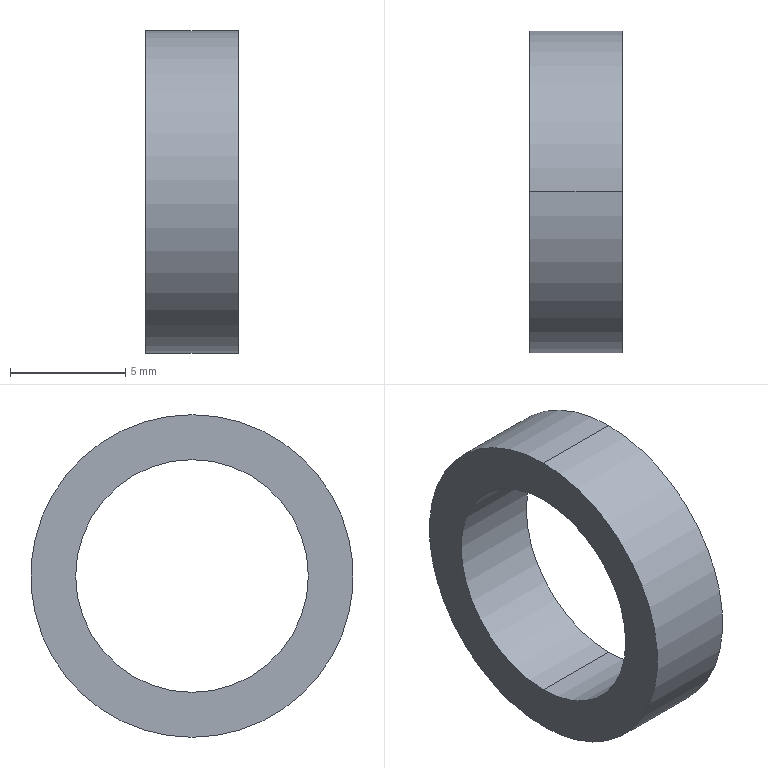Part | SolidWorks | features BaseBody 1 | 1 solid | 6 faces | box 4 x 14 x 14 mm | volume 295.278 mm3 | cylinder 4 | plane 2 | commonest cylinder face diameters 10.1 x2 14 x2
STEP:
#1=CARTESIAN_POINT('',(-2.,0.,-7.));
#2=VERTEX_POINT('',#1);
#3=CARTESIAN_POINT('',(-2.,0.,7.));
#4=VERTEX_POINT('',#3);
#5=CARTESIAN_POINT('',(-2.,0.,0.));
#6=DIRECTION('',(1.,0.,0.));
#7=DIRECTION('',(0.,0.,-1.));
#8=AXIS2_PLACEMENT_3D('',#5,#6,#7);
#9=CIRCLE('',#8,7.);
#10=EDGE_CURVE('',#2,#4,#9,.T.);
#11=ORIENTED_EDGE('',*,*,#10,.T.);
#12=CARTESIAN_POINT('',(2.,0.,7.));
#13=VERTEX_POINT('',#12);
#14=CARTESIAN_POINT('',(-2.,0.,7.));
#15=DIRECTION('',(1.,0.,0.));
#16=VECTOR('',#15,1000.);
#17=LINE('',#14,#16);
#18=EDGE_CURVE('',#4,#13,#17,.T.);
#19=ORIENTED_EDGE('',*,*,#18,.T.);
#20=CARTESIAN_POINT('',(2.,0.,-7.));
#21=VERTEX_POINT('',#20);
#22=CARTESIAN_POINT('',(2.,0.,0.));
#23=DIRECTION('',(-1.,0.,0.));
#24=DIRECTION('',(0.,0.,-1.));
#25=AXIS2_PLACEMENT_3D('',#22,#23,#24);
#26=CIRCLE('',#25,7.);
#27=EDGE_CURVE('',#13,#21,#26,.T.);
#28=ORIENTED_EDGE('',*,*,#27,.T.);
#29=CARTESIAN_POINT('',(-2.,0.,-7.));
#30=DIRECTION('',(1.,0.,0.));
#31=VECTOR('',#30,1000.);
#32=LINE('',#29,#31);
#33=EDGE_CURVE('',#2,#21,#32,.T.);
#34=ORIENTED_EDGE('',*,*,#33,.F.);
#35=EDGE_LOOP('',(#11,#19,#28,#34));
#36=FACE_OUTER_BOUND('',#35,.T.);
#37=CARTESIAN_POINT('',(-2.,0.,0.));
#38=DIRECTION('',(1.,0.,0.));
#39=DIRECTION('',(0.,0.,-1.));
#40=AXIS2_PLACEMENT_3D('',#37,#38,#39);
#41=CYLINDRICAL_SURFACE('',#40,7.);
#42=ADVANCED_FACE('',(#36),#41,.T.);
#43=CARTESIAN_POINT('',(-2.,0.,-5.05));
#44=VERTEX_POINT('',#43);
#45=CARTESIAN_POINT('',(-2.,0.,5.05));
#46=VERTEX_POINT('',#45);
#47=CARTESIAN_POINT('',(-2.,0.,0.));
#48=DIRECTION('',(-1.,0.,0.));
#49=DIRECTION('',(0.,0.,-1.));
#50=AXIS2_PLACEMENT_3D('',#47,#48,#49);
#51=CIRCLE('',#50,5.05);
#52=EDGE_CURVE('',#44,#46,#51,.T.);
#53=ORIENTED_EDGE('',*,*,#52,.T.);
#54=CARTESIAN_POINT('',(2.,0.,5.05));
#55=VERTEX_POINT('',#54);
#56=CARTESIAN_POINT('',(-3.,0.,5.05));
#57=DIRECTION('',(1.,0.,0.));
#58=VECTOR('',#57,1000.);
#59=LINE('',#56,#58);
#60=EDGE_CURVE('',#46,#55,#59,.T.);
#61=ORIENTED_EDGE('',*,*,#60,.T.);
#62=CARTESIAN_POINT('',(2.,0.,-5.05));
#63=VERTEX_POINT('',#62);
#64=CARTESIAN_POINT('',(2.,0.,0.));
#65=DIRECTION('',(-1.,0.,0.));
#66=DIRECTION('',(0.,0.,-1.));
#67=AXIS2_PLACEMENT_3D('',#64,#65,#66);
#68=CIRCLE('',#67,5.05);
#69=EDGE_CURVE('',#63,#55,#68,.T.);
#70=ORIENTED_EDGE('',*,*,#69,.F.);
#71=CARTESIAN_POINT('',(-3.,0.,-5.05));
#72=DIRECTION('',(1.,0.,0.));
#73=VECTOR('',#72,1000.);
#74=LINE('',#71,#73);
#75=EDGE_CURVE('',#44,#63,#74,.T.);
#76=ORIENTED_EDGE('',*,*,#75,.F.);
#77=EDGE_LOOP('',(#53,#61,#70,#76));
#78=FACE_OUTER_BOUND('',#77,.T.);
#79=CARTESIAN_POINT('',(-3.,0.,0.));
#80=DIRECTION('',(1.,0.,0.));
#81=DIRECTION('',(0.,0.,-1.));
#82=AXIS2_PLACEMENT_3D('',#79,#80,#81);
#83=CYLINDRICAL_SURFACE('',#82,5.05);
#84=ADVANCED_FACE('',(#78),#83,.F.);
#85=ORIENTED_EDGE('',*,*,#18,.F.);
#86=CARTESIAN_POINT('',(-2.,0.,0.));
#87=DIRECTION('',(1.,0.,0.));
#88=DIRECTION('',(0.,0.,-1.));
#89=AXIS2_PLACEMENT_3D('',#86,#87,#88);
#90=CIRCLE('',#89,7.);
#91=EDGE_CURVE('',#4,#2,#90,.T.);
#92=ORIENTED_EDGE('',*,*,#91,.T.);
#93=ORIENTED_EDGE('',*,*,#33,.T.);
#94=CARTESIAN_POINT('',(2.,0.,0.));
#95=DIRECTION('',(-1.,0.,0.));
#96=DIRECTION('',(0.,0.,-1.));
#97=AXIS2_PLACEMENT_3D('',#94,#95,#96);
#98=CIRCLE('',#97,7.);
#99=EDGE_CURVE('',#21,#13,#98,.T.);
#100=ORIENTED_EDGE('',*,*,#99,.T.);
#101=EDGE_LOOP('',(#85,#92,#93,#100));
#102=FACE_OUTER_BOUND('',#101,.T.);
#103=CARTESIAN_POINT('',(-2.,0.,0.));
#104=DIRECTION('',(1.,0.,0.));
#105=DIRECTION('',(0.,0.,-1.));
#106=AXIS2_PLACEMENT_3D('',#103,#104,#105);
#107=CYLINDRICAL_SURFACE('',#106,7.);
#108=ADVANCED_FACE('',(#102),#107,.T.);
#109=ORIENTED_EDGE('',*,*,#52,.F.);
#110=CARTESIAN_POINT('',(-2.,0.,0.));
#111=DIRECTION('',(-1.,0.,0.));
#112=DIRECTION('',(0.,0.,-1.));
#113=AXIS2_PLACEMENT_3D('',#110,#111,#112);
#114=CIRCLE('',#113,5.05);
#115=EDGE_CURVE('',#46,#44,#114,.T.);
#116=ORIENTED_EDGE('',*,*,#115,.F.);
#117=EDGE_LOOP('',(#109,#116));
#118=FACE_BOUND('',#117,.T.);
#119=ORIENTED_EDGE('',*,*,#10,.F.);
#120=ORIENTED_EDGE('',*,*,#91,.F.);
#121=EDGE_LOOP('',(#119,#120));
#122=FACE_OUTER_BOUND('',#121,.T.);
#123=CARTESIAN_POINT('',(-2.,0.,0.));
#124=DIRECTION('',(1.,0.,0.));
#125=DIRECTION('',(0.,0.,-1.));
#126=AXIS2_PLACEMENT_3D('',#123,#124,#125);
#127=PLANE('',#126);
#128=ADVANCED_FACE('',(#118,#122),#127,.F.);
#129=ORIENTED_EDGE('',*,*,#69,.T.);
#130=CARTESIAN_POINT('',(2.,0.,0.));
#131=DIRECTION('',(-1.,0.,0.));
#132=DIRECTION('',(0.,0.,-1.));
#133=AXIS2_PLACEMENT_3D('',#130,#131,#132);
#134=CIRCLE('',#133,5.05);
#135=EDGE_CURVE('',#55,#63,#134,.T.);
#136=ORIENTED_EDGE('',*,*,#135,.T.);
#137=EDGE_LOOP('',(#129,#136));
#138=FACE_BOUND('',#137,.T.);
#139=ORIENTED_EDGE('',*,*,#99,.F.);
#140=ORIENTED_EDGE('',*,*,#27,.F.);
#141=EDGE_LOOP('',(#139,#140));
#142=FACE_OUTER_BOUND('',#141,.T.);
#143=CARTESIAN_POINT('',(2.,0.,0.));
#144=DIRECTION('',(1.,0.,0.));
#145=DIRECTION('',(0.,0.,-1.));
#146=AXIS2_PLACEMENT_3D('',#143,#144,#145);
#147=PLANE('',#146);
#148=ADVANCED_FACE('',(#138,#142),#147,.T.);
#149=ORIENTED_EDGE('',*,*,#60,.F.);
#150=ORIENTED_EDGE('',*,*,#115,.T.);
#151=ORIENTED_EDGE('',*,*,#75,.T.);
#152=ORIENTED_EDGE('',*,*,#135,.F.);
#153=EDGE_LOOP('',(#149,#150,#151,#152));
#154=FACE_OUTER_BOUND('',#153,.T.);
#155=CARTESIAN_POINT('',(-3.,0.,0.));
#156=DIRECTION('',(1.,0.,0.));
#157=DIRECTION('',(0.,0.,-1.));
#158=AXIS2_PLACEMENT_3D('',#155,#156,#157);
#159=CYLINDRICAL_SURFACE('',#158,5.05);
#160=ADVANCED_FACE('',(#154),#159,.F.);
#161=CLOSED_SHELL('',(#42,#84,#108,#128,#148,#160));
#162=MANIFOLD_SOLID_BREP('',#161);
#163=CARTESIAN_POINT('',(0.,0.,0.));
#164=DIRECTION('',(0.,0.,1.));
#165=DIRECTION('',(1.,0.,0.));
#166=AXIS2_PLACEMENT_3D('',#163,#164,#165);
#167=(LENGTH_UNIT()NAMED_UNIT(*)SI_UNIT(.MILLI.,.METRE.));
#168=UNCERTAINTY_MEASURE_WITH_UNIT(LENGTH_MEASURE(0.00001),#167,'','');
#169=(NAMED_UNIT(*)PLANE_ANGLE_UNIT()SI_UNIT($,.RADIAN.));
#170=(NAMED_UNIT(*)SI_UNIT($,.STERADIAN.)SOLID_ANGLE_UNIT());
#171=(GEOMETRIC_REPRESENTATION_CONTEXT(3)GLOBAL_UNCERTAINTY_ASSIGNED_CONTEXT((#168))GLOBAL_UNIT_ASSIGNED_CONTEXT((#167,#169,#170))REPRESENTATION_CONTEXT('',''));
#172=ADVANCED_BREP_SHAPE_REPRESENTATION('',(#162,#166),#171);